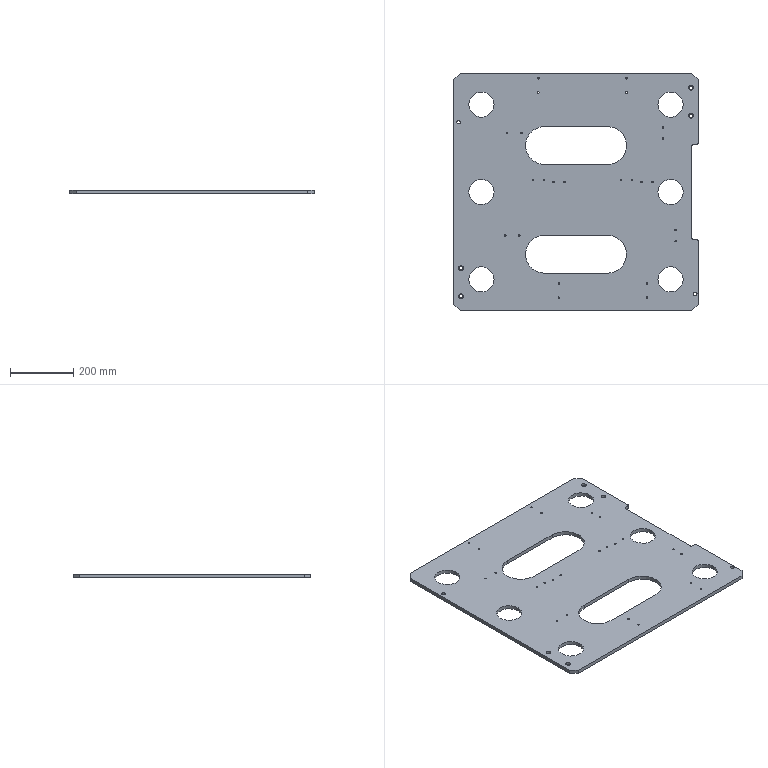Part | SolidWorks | features Cut 2, HoleWzd 2, ICE 2, Chamfer 1, Extrusion 1, Fillet 1 | 1 solid | 680 faces | box 775 x 755 x 12 mm | volume 5715075 mm3 | plane 426 | spline 164 | cylinder 90 | commonest cylinder face diameters 5 x48 80 x12 9 x8 15 x8 120 x6 10 x4